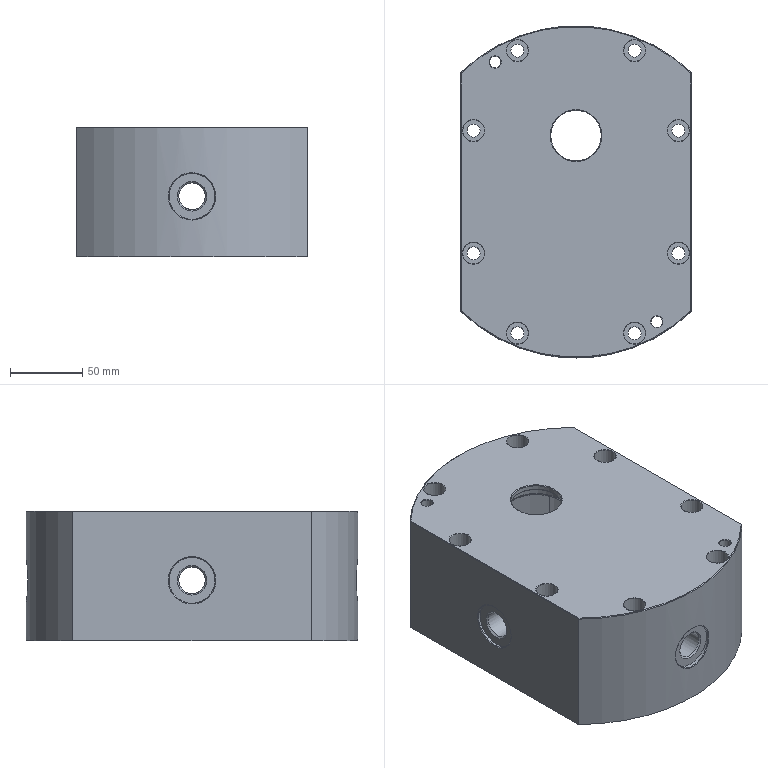Part | 1 solid | 99 faces | box 160 x 230 x 90 mm | volume 1331346 mm3 | cylinder 48 | plane 28 | cone 21 | spline 2 | commonest cylinder face diameters 9 x8 15 x8 18.5 x4 30 x4 32 x4 36 x4